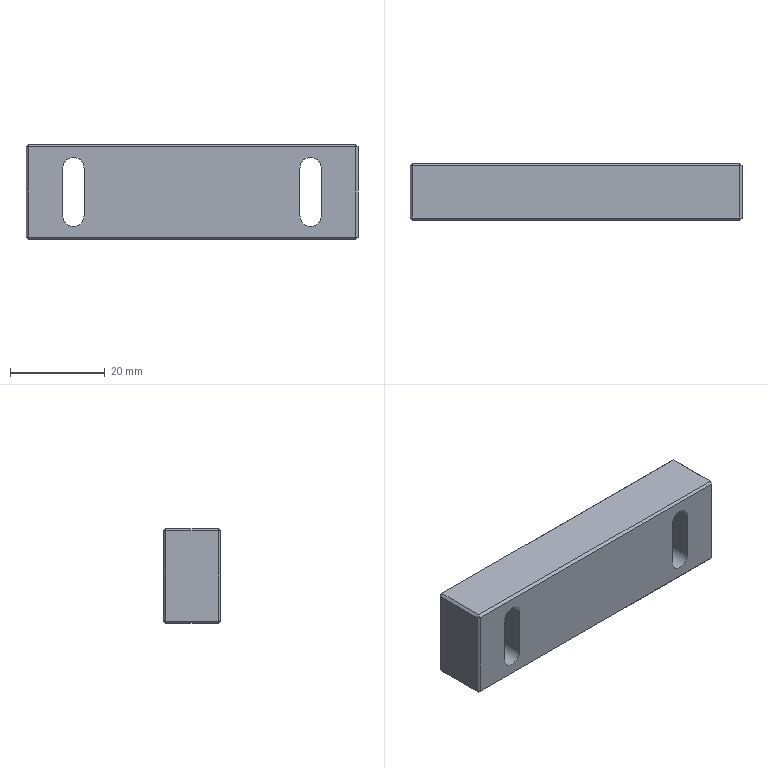Part | SolidWorks | features Chamfer 1, Cut 1, Extrusion 1 | 1 solid | 36 faces | box 70 x 12 x 20 mm | volume 15288 mm3 | plane 30 | cylinder 6 | commonest cylinder face diameters 4.5 x6
STEP:
#1=CARTESIAN_POINT('',(25.,0.,7.25));
#2=VERTEX_POINT('',#1);
#3=CARTESIAN_POINT('',(27.25,0.,5.));
#4=VERTEX_POINT('',#3);
#5=CARTESIAN_POINT('',(25.,0.,5.));
#6=DIRECTION('',(0.,1.,0.));
#7=DIRECTION('',(0.,0.,1.));
#8=AXIS2_PLACEMENT_3D('',#5,#6,#7);
#9=CIRCLE('',#8,2.25);
#10=EDGE_CURVE('',#2,#4,#9,.T.);
#11=ORIENTED_EDGE('',*,*,#10,.F.);
#12=CARTESIAN_POINT('',(25.,12.,7.25));
#13=VERTEX_POINT('',#12);
#14=CARTESIAN_POINT('',(25.,0.,7.25));
#15=DIRECTION('',(0.,1.,0.));
#16=VECTOR('',#15,1000.);
#17=LINE('',#14,#16);
#18=EDGE_CURVE('',#2,#13,#17,.T.);
#19=ORIENTED_EDGE('',*,*,#18,.T.);
#20=CARTESIAN_POINT('',(27.25,12.,5.));
#21=VERTEX_POINT('',#20);
#22=CARTESIAN_POINT('',(25.,12.,5.));
#23=DIRECTION('',(0.,1.,0.));
#24=DIRECTION('',(0.,0.,1.));
#25=AXIS2_PLACEMENT_3D('',#22,#23,#24);
#26=CIRCLE('',#25,2.25);
#27=EDGE_CURVE('',#13,#21,#26,.T.);
#28=ORIENTED_EDGE('',*,*,#27,.T.);
#29=CARTESIAN_POINT('',(27.25,0.,5.));
#30=DIRECTION('',(0.,1.,0.));
#31=VECTOR('',#30,1000.);
#32=LINE('',#29,#31);
#33=EDGE_CURVE('',#4,#21,#32,.T.);
#34=ORIENTED_EDGE('',*,*,#33,.F.);
#35=EDGE_LOOP('',(#11,#19,#28,#34));
#36=FACE_OUTER_BOUND('',#35,.T.);
#37=CARTESIAN_POINT('',(25.,0.,5.));
#38=DIRECTION('',(0.,1.,0.));
#39=DIRECTION('',(0.,0.,1.));
#40=AXIS2_PLACEMENT_3D('',#37,#38,#39);
#41=CYLINDRICAL_SURFACE('',#40,2.25);
#42=ADVANCED_FACE('',(#36),#41,.F.);
#43=CARTESIAN_POINT('',(-25.,0.,7.25));
#44=VERTEX_POINT('',#43);
#45=CARTESIAN_POINT('',(-22.75,0.,5.));
#46=VERTEX_POINT('',#45);
#47=CARTESIAN_POINT('',(-25.,0.,5.));
#48=DIRECTION('',(0.,1.,0.));
#49=DIRECTION('',(0.,0.,-1.));
#50=AXIS2_PLACEMENT_3D('',#47,#48,#49);
#51=CIRCLE('',#50,2.25);
#52=EDGE_CURVE('',#44,#46,#51,.T.);
#53=ORIENTED_EDGE('',*,*,#52,.F.);
#54=CARTESIAN_POINT('',(-25.,12.,7.25));
#55=VERTEX_POINT('',#54);
#56=CARTESIAN_POINT('',(-25.,0.,7.25));
#57=DIRECTION('',(0.,1.,0.));
#58=VECTOR('',#57,1000.);
#59=LINE('',#56,#58);
#60=EDGE_CURVE('',#44,#55,#59,.T.);
#61=ORIENTED_EDGE('',*,*,#60,.T.);
#62=CARTESIAN_POINT('',(-22.75,12.,5.));
#63=VERTEX_POINT('',#62);
#64=CARTESIAN_POINT('',(-25.,12.,5.));
#65=DIRECTION('',(0.,1.,0.));
#66=DIRECTION('',(0.,0.,-1.));
#67=AXIS2_PLACEMENT_3D('',#64,#65,#66);
#68=CIRCLE('',#67,2.25);
#69=EDGE_CURVE('',#55,#63,#68,.T.);
#70=ORIENTED_EDGE('',*,*,#69,.T.);
#71=CARTESIAN_POINT('',(-22.75,0.,5.));
#72=DIRECTION('',(0.,1.,0.));
#73=VECTOR('',#72,1000.);
#74=LINE('',#71,#73);
#75=EDGE_CURVE('',#46,#63,#74,.T.);
#76=ORIENTED_EDGE('',*,*,#75,.F.);
#77=EDGE_LOOP('',(#53,#61,#70,#76));
#78=FACE_OUTER_BOUND('',#77,.T.);
#79=CARTESIAN_POINT('',(-25.,0.,5.));
#80=DIRECTION('',(0.,1.,0.));
#81=DIRECTION('',(0.,0.,1.));
#82=AXIS2_PLACEMENT_3D('',#79,#80,#81);
#83=CYLINDRICAL_SURFACE('',#82,2.25);
#84=ADVANCED_FACE('',(#78),#83,.F.);
#85=CARTESIAN_POINT('',(-35.,11.5,9.5));
#86=VERTEX_POINT('',#85);
#87=CARTESIAN_POINT('',(-35.,11.5,-9.5));
#88=VERTEX_POINT('',#87);
#89=CARTESIAN_POINT('',(-35.,11.5,-10.));
#90=DIRECTION('',(0.,0.,-1.));
#91=VECTOR('',#90,1000.);
#92=LINE('',#89,#91);
#93=EDGE_CURVE('',#86,#88,#92,.T.);
#94=ORIENTED_EDGE('',*,*,#93,.T.);
#95=CARTESIAN_POINT('',(-35.,0.5,-9.5));
#96=VERTEX_POINT('',#95);
#97=CARTESIAN_POINT('',(-35.,12.,-9.5));
#98=DIRECTION('',(0.,-1.,0.));
#99=VECTOR('',#98,1000.);
#100=LINE('',#97,#99);
#101=EDGE_CURVE('',#88,#96,#100,.T.);
#102=ORIENTED_EDGE('',*,*,#101,.T.);
#103=CARTESIAN_POINT('',(-35.,0.5,9.5));
#104=VERTEX_POINT('',#103);
#105=CARTESIAN_POINT('',(-35.,0.5,-10.));
#106=DIRECTION('',(0.,0.,1.));
#107=VECTOR('',#106,1000.);
#108=LINE('',#105,#107);
#109=EDGE_CURVE('',#96,#104,#108,.T.);
#110=ORIENTED_EDGE('',*,*,#109,.T.);
#111=CARTESIAN_POINT('',(-35.,12.,9.5));
#112=DIRECTION('',(0.,1.,0.));
#113=VECTOR('',#112,1000.);
#114=LINE('',#111,#113);
#115=EDGE_CURVE('',#104,#86,#114,.T.);
#116=ORIENTED_EDGE('',*,*,#115,.T.);
#117=EDGE_LOOP('',(#94,#102,#110,#116));
#118=FACE_OUTER_BOUND('',#117,.T.);
#119=CARTESIAN_POINT('',(-35.,12.,-10.));
#120=DIRECTION('',(1.,0.,0.));
#121=DIRECTION('',(0.,0.,-1.));
#122=AXIS2_PLACEMENT_3D('',#119,#120,#121);
#123=PLANE('',#122);
#124=ADVANCED_FACE('',(#118),#123,.F.);
#125=CARTESIAN_POINT('',(-34.5,0.5,10.));
#126=VERTEX_POINT('',#125);
#127=CARTESIAN_POINT('',(34.5,0.5,10.));
#128=VERTEX_POINT('',#127);
#129=CARTESIAN_POINT('',(-35.,0.5,10.));
#130=DIRECTION('',(1.,0.,0.));
#131=VECTOR('',#130,1000.);
#132=LINE('',#129,#131);
#133=EDGE_CURVE('',#126,#128,#132,.T.);
#134=ORIENTED_EDGE('',*,*,#133,.T.);
#135=CARTESIAN_POINT('',(34.5,11.5,10.));
#136=VERTEX_POINT('',#135);
#137=CARTESIAN_POINT('',(34.5,12.,10.));
#138=DIRECTION('',(0.,1.,0.));
#139=VECTOR('',#138,1000.);
#140=LINE('',#137,#139);
#141=EDGE_CURVE('',#128,#136,#140,.T.);
#142=ORIENTED_EDGE('',*,*,#141,.T.);
#143=CARTESIAN_POINT('',(-34.5,11.5,10.));
#144=VERTEX_POINT('',#143);
#145=CARTESIAN_POINT('',(-35.,11.5,10.));
#146=DIRECTION('',(-1.,0.,0.));
#147=VECTOR('',#146,1000.);
#148=LINE('',#145,#147);
#149=EDGE_CURVE('',#136,#144,#148,.T.);
#150=ORIENTED_EDGE('',*,*,#149,.T.);
#151=CARTESIAN_POINT('',(-34.5,12.,10.));
#152=DIRECTION('',(0.,-1.,0.));
#153=VECTOR('',#152,1000.);
#154=LINE('',#151,#153);
#155=EDGE_CURVE('',#144,#126,#154,.T.);
#156=ORIENTED_EDGE('',*,*,#155,.T.);
#157=EDGE_LOOP('',(#134,#142,#150,#156));
#158=FACE_OUTER_BOUND('',#157,.T.);
#159=CARTESIAN_POINT('',(-35.,12.,10.));
#160=DIRECTION('',(0.,0.,-1.));
#161=DIRECTION('',(-1.,0.,0.));
#162=AXIS2_PLACEMENT_3D('',#159,#160,#161);
#163=PLANE('',#162);
#164=ADVANCED_FACE('',(#158),#163,.F.);
#165=CARTESIAN_POINT('',(35.,11.5,-9.5));
#166=VERTEX_POINT('',#165);
#167=CARTESIAN_POINT('',(35.,11.5,9.5));
#168=VERTEX_POINT('',#167);
#169=CARTESIAN_POINT('',(35.,11.5,10.));
#170=DIRECTION('',(0.,0.,1.));
#171=VECTOR('',#170,1000.);
#172=LINE('',#169,#171);
#173=EDGE_CURVE('',#166,#168,#172,.T.);
#174=ORIENTED_EDGE('',*,*,#173,.T.);
#175=CARTESIAN_POINT('',(35.,0.5,9.5));
#176=VERTEX_POINT('',#175);
#177=CARTESIAN_POINT('',(35.,12.,9.5));
#178=DIRECTION('',(0.,-1.,0.));
#179=VECTOR('',#178,1000.);
#180=LINE('',#177,#179);
#181=EDGE_CURVE('',#168,#176,#180,.T.);
#182=ORIENTED_EDGE('',*,*,#181,.T.);
#183=CARTESIAN_POINT('',(35.,0.5,-9.5));
#184=VERTEX_POINT('',#183);
#185=CARTESIAN_POINT('',(35.,0.5,-10.));
#186=DIRECTION('',(0.,0.,-1.));
#187=VECTOR('',#186,1000.);
#188=LINE('',#185,#187);
#189=EDGE_CURVE('',#176,#184,#188,.T.);
#190=ORIENTED_EDGE('',*,*,#189,.T.);
#191=CARTESIAN_POINT('',(35.,12.,-9.5));
#192=DIRECTION('',(0.,1.,0.));
#193=VECTOR('',#192,1000.);
#194=LINE('',#191,#193);
#195=EDGE_CURVE('',#184,#166,#194,.T.);
#196=ORIENTED_EDGE('',*,*,#195,.T.);
#197=EDGE_LOOP('',(#174,#182,#190,#196));
#198=FACE_OUTER_BOUND('',#197,.T.);
#199=CARTESIAN_POINT('',(35.,12.,-10.));
#200=DIRECTION('',(-1.,0.,0.));
#201=DIRECTION('',(0.,0.,1.));
#202=AXIS2_PLACEMENT_3D('',#199,#200,#201);
#203=PLANE('',#202);
#204=ADVANCED_FACE('',(#198),#203,.F.);
#205=CARTESIAN_POINT('',(-34.5,11.5,-10.));
#206=VERTEX_POINT('',#205);
#207=CARTESIAN_POINT('',(34.5,11.5,-10.));
#208=VERTEX_POINT('',#207);
#209=CARTESIAN_POINT('',(35.,11.5,-10.));
#210=DIRECTION('',(1.,0.,0.));
#211=VECTOR('',#210,1000.);
#212=LINE('',#209,#211);
#213=EDGE_CURVE('',#206,#208,#212,.T.);
#214=ORIENTED_EDGE('',*,*,#213,.T.);
#215=CARTESIAN_POINT('',(34.5,0.5,-10.));
#216=VERTEX_POINT('',#215);
#217=CARTESIAN_POINT('',(34.5,12.,-10.));
#218=DIRECTION('',(0.,-1.,0.));
#219=VECTOR('',#218,1000.);
#220=LINE('',#217,#219);
#221=EDGE_CURVE('',#208,#216,#220,.T.);
#222=ORIENTED_EDGE('',*,*,#221,.T.);
#223=CARTESIAN_POINT('',(-34.5,0.5,-10.));
#224=VERTEX_POINT('',#223);
#225=CARTESIAN_POINT('',(-35.,0.5,-10.));
#226=DIRECTION('',(-1.,0.,0.));
#227=VECTOR('',#226,1000.);
#228=LINE('',#225,#227);
#229=EDGE_CURVE('',#216,#224,#228,.T.);
#230=ORIENTED_EDGE('',*,*,#229,.T.);
#231=CARTESIAN_POINT('',(-34.5,12.,-10.));
#232=DIRECTION('',(0.,1.,0.));
#233=VECTOR('',#232,1000.);
#234=LINE('',#231,#233);
#235=EDGE_CURVE('',#224,#206,#234,.T.);
#236=ORIENTED_EDGE('',*,*,#235,.T.);
#237=EDGE_LOOP('',(#214,#222,#230,#236));
#238=FACE_OUTER_BOUND('',#237,.T.);
#239=CARTESIAN_POINT('',(-35.,12.,-10.));
#240=DIRECTION('',(0.,0.,1.));
#241=DIRECTION('',(1.,0.,0.));
#242=AXIS2_PLACEMENT_3D('',#239,#240,#241);
#243=PLANE('',#242);
#244=ADVANCED_FACE('',(#238),#243,.F.);
#245=CARTESIAN_POINT('',(-34.5,12.,-9.5));
#246=VERTEX_POINT('',#245);
#247=CARTESIAN_POINT('',(-34.5,12.,9.5));
#248=VERTEX_POINT('',#247);
#249=CARTESIAN_POINT('',(-34.5,12.,10.));
#250=DIRECTION('',(0.,0.,1.));
#251=VECTOR('',#250,1000.);
#252=LINE('',#249,#251);
#253=EDGE_CURVE('',#246,#248,#252,.T.);
#254=ORIENTED_EDGE('',*,*,#253,.T.);
#255=CARTESIAN_POINT('',(34.5,12.,9.5));
#256=VERTEX_POINT('',#255);
#257=CARTESIAN_POINT('',(35.,12.,9.5));
#258=DIRECTION('',(1.,0.,0.));
#259=VECTOR('',#258,1000.);
#260=LINE('',#257,#259);
#261=EDGE_CURVE('',#248,#256,#260,.T.);
#262=ORIENTED_EDGE('',*,*,#261,.T.);
#263=CARTESIAN_POINT('',(34.5,12.,-9.5));
#264=VERTEX_POINT('',#263);
#265=CARTESIAN_POINT('',(34.5,12.,-10.));
#266=DIRECTION('',(0.,0.,-1.));
#267=VECTOR('',#266,1000.);
#268=LINE('',#265,#267);
#269=EDGE_CURVE('',#256,#264,#268,.T.);
#270=ORIENTED_EDGE('',*,*,#269,.T.);
#271=CARTESIAN_POINT('',(-35.,12.,-9.5));
#272=DIRECTION('',(-1.,0.,0.));
#273=VECTOR('',#272,1000.);
#274=LINE('',#271,#273);
#275=EDGE_CURVE('',#264,#246,#274,.T.);
#276=ORIENTED_EDGE('',*,*,#275,.T.);
#277=EDGE_LOOP('',(#254,#262,#270,#276));
#278=FACE_OUTER_BOUND('',#277,.T.);
#279=CARTESIAN_POINT('',(22.75,12.,5.));
#280=VERTEX_POINT('',#279);
#281=CARTESIAN_POINT('',(25.,12.,5.));
#282=DIRECTION('',(0.,1.,0.));
#283=DIRECTION('',(0.,0.,1.));
#284=AXIS2_PLACEMENT_3D('',#281,#282,#283);
#285=CIRCLE('',#284,2.25);
#286=EDGE_CURVE('',#280,#13,#285,.T.);
#287=ORIENTED_EDGE('',*,*,#286,.F.);
#288=CARTESIAN_POINT('',(22.75,12.,-5.));
#289=VERTEX_POINT('',#288);
#290=CARTESIAN_POINT('',(22.75,12.,-5.));
#291=DIRECTION('',(0.,0.,1.));
#292=VECTOR('',#291,1000.);
#293=LINE('',#290,#292);
#294=EDGE_CURVE('',#289,#280,#293,.T.);
#295=ORIENTED_EDGE('',*,*,#294,.F.);
#296=CARTESIAN_POINT('',(27.25,12.,-5.));
#297=VERTEX_POINT('',#296);
#298=CARTESIAN_POINT('',(25.,12.,-5.));
#299=DIRECTION('',(0.,1.,0.));
#300=DIRECTION('',(0.,0.,1.));
#301=AXIS2_PLACEMENT_3D('',#298,#299,#300);
#302=CIRCLE('',#301,2.25);
#303=EDGE_CURVE('',#297,#289,#302,.T.);
#304=ORIENTED_EDGE('',*,*,#303,.F.);
#305=CARTESIAN_POINT('',(27.25,12.,-5.));
#306=DIRECTION('',(0.,0.,-1.));
#307=VECTOR('',#306,1000.);
#308=LINE('',#305,#307);
#309=EDGE_CURVE('',#21,#297,#308,.T.);
#310=ORIENTED_EDGE('',*,*,#309,.F.);
#311=ORIENTED_EDGE('',*,*,#27,.F.);
#312=EDGE_LOOP('',(#287,#295,#304,#310,#311));
#313=FACE_BOUND('',#312,.T.);
#314=CARTESIAN_POINT('',(-22.75,12.,-5.));
#315=VERTEX_POINT('',#314);
#316=CARTESIAN_POINT('',(-27.25,12.,-5.));
#317=VERTEX_POINT('',#316);
#318=CARTESIAN_POINT('',(-25.,12.,-5.));
#319=DIRECTION('',(0.,1.,0.));
#320=DIRECTION('',(0.,0.,-1.));
#321=AXIS2_PLACEMENT_3D('',#318,#319,#320);
#322=CIRCLE('',#321,2.25);
#323=EDGE_CURVE('',#315,#317,#322,.T.);
#324=ORIENTED_EDGE('',*,*,#323,.F.);
#325=CARTESIAN_POINT('',(-22.75,12.,-5.));
#326=DIRECTION('',(0.,0.,-1.));
#327=VECTOR('',#326,1000.);
#328=LINE('',#325,#327);
#329=EDGE_CURVE('',#63,#315,#328,.T.);
#330=ORIENTED_EDGE('',*,*,#329,.F.);
#331=ORIENTED_EDGE('',*,*,#69,.F.);
#332=CARTESIAN_POINT('',(-27.25,12.,5.));
#333=VERTEX_POINT('',#332);
#334=CARTESIAN_POINT('',(-25.,12.,5.));
#335=DIRECTION('',(0.,1.,0.));
#336=DIRECTION('',(0.,0.,-1.));
#337=AXIS2_PLACEMENT_3D('',#334,#335,#336);
#338=CIRCLE('',#337,2.25);
#339=EDGE_CURVE('',#333,#55,#338,.T.);
#340=ORIENTED_EDGE('',*,*,#339,.F.);
#341=CARTESIAN_POINT('',(-27.25,12.,-5.));
#342=DIRECTION('',(0.,0.,1.));
#343=VECTOR('',#342,1000.);
#344=LINE('',#341,#343);
#345=EDGE_CURVE('',#317,#333,#344,.T.);
#346=ORIENTED_EDGE('',*,*,#345,.F.);
#347=EDGE_LOOP('',(#324,#330,#331,#340,#346));
#348=FACE_BOUND('',#347,.T.);
#349=CARTESIAN_POINT('',(-35.,12.,10.));
#350=DIRECTION('',(0.,1.,0.));
#351=DIRECTION('',(0.,0.,1.));
#352=AXIS2_PLACEMENT_3D('',#349,#350,#351);
#353=PLANE('',#352);
#354=ADVANCED_FACE('',(#278,#313,#348),#353,.T.);
#355=CARTESIAN_POINT('',(34.5,0.,-9.5));
#356=VERTEX_POINT('',#355);
#357=CARTESIAN_POINT('',(34.5,0.,9.5));
#358=VERTEX_POINT('',#357);
#359=CARTESIAN_POINT('',(34.5,0.,10.));
#360=DIRECTION('',(0.,0.,1.));
#361=VECTOR('',#360,1000.);
#362=LINE('',#359,#361);
#363=EDGE_CURVE('',#356,#358,#362,.T.);
#364=ORIENTED_EDGE('',*,*,#363,.T.);
#365=CARTESIAN_POINT('',(-34.5,0.,9.5));
#366=VERTEX_POINT('',#365);
#367=CARTESIAN_POINT('',(-35.,0.,9.5));
#368=DIRECTION('',(-1.,0.,0.));
#369=VECTOR('',#368,1000.);
#370=LINE('',#367,#369);
#371=EDGE_CURVE('',#358,#366,#370,.T.);
#372=ORIENTED_EDGE('',*,*,#371,.T.);
#373=CARTESIAN_POINT('',(-34.5,0.,-9.5));
#374=VERTEX_POINT('',#373);
#375=CARTESIAN_POINT('',(-34.5,0.,10.));
#376=DIRECTION('',(0.,0.,-1.));
#377=VECTOR('',#376,1000.);
#378=LINE('',#375,#377);
#379=EDGE_CURVE('',#366,#374,#378,.T.);
#380=ORIENTED_EDGE('',*,*,#379,.T.);
#381=CARTESIAN_POINT('',(-35.,0.,-9.5));
#382=DIRECTION('',(1.,0.,0.));
#383=VECTOR('',#382,1000.);
#384=LINE('',#381,#383);
#385=EDGE_CURVE('',#374,#356,#384,.T.);
#386=ORIENTED_EDGE('',*,*,#385,.T.);
#387=EDGE_LOOP('',(#364,#372,#380,#386));
#388=FACE_OUTER_BOUND('',#387,.T.);
#389=CARTESIAN_POINT('',(22.75,0.,-5.));
#390=VERTEX_POINT('',#389);
#391=CARTESIAN_POINT('',(22.75,0.,5.));
#392=VERTEX_POINT('',#391);
#393=CARTESIAN_POINT('',(22.75,0.,-5.));
#394=DIRECTION('',(0.,0.,1.));
#395=VECTOR('',#394,1000.);
#396=LINE('',#393,#395);
#397=EDGE_CURVE('',#390,#392,#396,.T.);
#398=ORIENTED_EDGE('',*,*,#397,.T.);
#399=CARTESIAN_POINT('',(25.,0.,5.));
#400=DIRECTION('',(0.,1.,0.));
#401=DIRECTION('',(0.,0.,1.));
#402=AXIS2_PLACEMENT_3D('',#399,#400,#401);
#403=CIRCLE('',#402,2.25);
#404=EDGE_CURVE('',#392,#2,#403,.T.);
#405=ORIENTED_EDGE('',*,*,#404,.T.);
#406=ORIENTED_EDGE('',*,*,#10,.T.);
#407=CARTESIAN_POINT('',(27.25,0.,-5.));
#408=VERTEX_POINT('',#407);
#409=CARTESIAN_POINT('',(27.25,0.,-5.));
#410=DIRECTION('',(0.,0.,-1.));
#411=VECTOR('',#410,1000.);
#412=LINE('',#409,#411);
#413=EDGE_CURVE('',#4,#408,#412,.T.);
#414=ORIENTED_EDGE('',*,*,#413,.T.);
#415=CARTESIAN_POINT('',(25.,0.,-5.));
#416=DIRECTION('',(0.,1.,0.));
#417=DIRECTION('',(0.,0.,1.));
#418=AXIS2_PLACEMENT_3D('',#415,#416,#417);
#419=CIRCLE('',#418,2.25);
#420=EDGE_CURVE('',#408,#390,#419,.T.);
#421=ORIENTED_EDGE('',*,*,#420,.T.);
#422=EDGE_LOOP('',(#398,#405,#406,#414,#421));
#423=FACE_BOUND('',#422,.T.);
#424=CARTESIAN_POINT('',(-22.75,0.,-5.));
#425=VERTEX_POINT('',#424);
#426=CARTESIAN_POINT('',(-22.75,0.,-5.));
#427=DIRECTION('',(0.,0.,-1.));
#428=VECTOR('',#427,1000.);
#429=LINE('',#426,#428);
#430=EDGE_CURVE('',#46,#425,#429,.T.);
#431=ORIENTED_EDGE('',*,*,#430,.T.);
#432=CARTESIAN_POINT('',(-27.25,0.,-5.));
#433=VERTEX_POINT('',#432);
#434=CARTESIAN_POINT('',(-25.,0.,-5.));
#435=DIRECTION('',(0.,1.,0.));
#436=DIRECTION('',(0.,0.,-1.));
#437=AXIS2_PLACEMENT_3D('',#434,#435,#436);
#438=CIRCLE('',#437,2.25);
#439=EDGE_CURVE('',#425,#433,#438,.T.);
#440=ORIENTED_EDGE('',*,*,#439,.T.);
#441=CARTESIAN_POINT('',(-27.25,0.,5.));
#442=VERTEX_POINT('',#441);
#443=CARTESIAN_POINT('',(-27.25,0.,-5.));
#444=DIRECTION('',(0.,0.,1.));
#445=VECTOR('',#444,1000.);
#446=LINE('',#443,#445);
#447=EDGE_CURVE('',#433,#442,#446,.T.);
#448=ORIENTED_EDGE('',*,*,#447,.T.);
#449=CARTESIAN_POINT('',(-25.,0.,5.));
#450=DIRECTION('',(0.,1.,0.));
#451=DIRECTION('',(0.,0.,-1.));
#452=AXIS2_PLACEMENT_3D('',#449,#450,#451);
#453=CIRCLE('',#452,2.25);
#454=EDGE_CURVE('',#442,#44,#453,.T.);
#455=ORIENTED_EDGE('',*,*,#454,.T.);
#456=ORIENTED_EDGE('',*,*,#52,.T.);
#457=EDGE_LOOP('',(#431,#440,#448,#455,#456));
#458=FACE_BOUND('',#457,.T.);
#459=CARTESIAN_POINT('',(-35.,0.,10.));
#460=DIRECTION('',(0.,1.,0.));
#461=DIRECTION('',(0.,0.,1.));
#462=AXIS2_PLACEMENT_3D('',#459,#460,#461);
#463=PLANE('',#462);
#464=ADVANCED_FACE('',(#388,#423,#458),#463,.F.);
#465=ORIENTED_EDGE('',*,*,#323,.T.);
#466=CARTESIAN_POINT('',(-27.25,0.,-5.));
#467=DIRECTION('',(0.,1.,0.));
#468=VECTOR('',#467,1000.);
#469=LINE('',#466,#468);
#470=EDGE_CURVE('',#433,#317,#469,.T.);
#471=ORIENTED_EDGE('',*,*,#470,.F.);
#472=ORIENTED_EDGE('',*,*,#439,.F.);
#473=CARTESIAN_POINT('',(-22.75,0.,-5.));
#474=DIRECTION('',(0.,1.,0.));
#475=VECTOR('',#474,1000.);
#476=LINE('',#473,#475);
#477=EDGE_CURVE('',#425,#315,#476,.T.);
#478=ORIENTED_EDGE('',*,*,#477,.T.);
#479=EDGE_LOOP('',(#465,#471,#472,#478));
#480=FACE_OUTER_BOUND('',#479,.T.);
#481=CARTESIAN_POINT('',(-25.,0.,-5.));
#482=DIRECTION('',(0.,1.,0.));
#483=DIRECTION('',(0.,0.,1.));
#484=AXIS2_PLACEMENT_3D('',#481,#482,#483);
#485=CYLINDRICAL_SURFACE('',#484,2.25);
#486=ADVANCED_FACE('',(#480),#485,.F.);
#487=ORIENTED_EDGE('',*,*,#329,.T.);
#488=ORIENTED_EDGE('',*,*,#477,.F.);
#489=ORIENTED_EDGE('',*,*,#430,.F.);
#490=ORIENTED_EDGE('',*,*,#75,.T.);
#491=EDGE_LOOP('',(#487,#488,#489,#490));
#492=FACE_OUTER_BOUND('',#491,.T.);
#493=CARTESIAN_POINT('',(-22.75,0.,-5.));
#494=DIRECTION('',(1.,0.,0.));
#495=DIRECTION('',(0.,0.,-1.));
#496=AXIS2_PLACEMENT_3D('',#493,#494,#495);
#497=PLANE('',#496);
#498=ADVANCED_FACE('',(#492),#497,.F.);
#499=ORIENTED_EDGE('',*,*,#60,.F.);
#500=ORIENTED_EDGE('',*,*,#454,.F.);
#501=CARTESIAN_POINT('',(-27.25,0.,5.));
#502=DIRECTION('',(0.,1.,0.));
#503=VECTOR('',#502,1000.);
#504=LINE('',#501,#503);
#505=EDGE_CURVE('',#442,#333,#504,.T.);
#506=ORIENTED_EDGE('',*,*,#505,.T.);
#507=ORIENTED_EDGE('',*,*,#339,.T.);
#508=EDGE_LOOP('',(#499,#500,#506,#507));
#509=FACE_OUTER_BOUND('',#508,.T.);
#510=CARTESIAN_POINT('',(-25.,0.,5.));
#511=DIRECTION('',(0.,1.,0.));
#512=DIRECTION('',(0.,0.,1.));
#513=AXIS2_PLACEMENT_3D('',#510,#511,#512);
#514=CYLINDRICAL_SURFACE('',#513,2.25);
#515=ADVANCED_FACE('',(#509),#514,.F.);
#516=ORIENTED_EDGE('',*,*,#345,.T.);
#517=ORIENTED_EDGE('',*,*,#505,.F.);
#518=ORIENTED_EDGE('',*,*,#447,.F.);
#519=ORIENTED_EDGE('',*,*,#470,.T.);
#520=EDGE_LOOP('',(#516,#517,#518,#519));
#521=FACE_OUTER_BOUND('',#520,.T.);
#522=CARTESIAN_POINT('',(-27.25,0.,-5.));
#523=DIRECTION('',(-1.,0.,0.));
#524=DIRECTION('',(0.,0.,1.));
#525=AXIS2_PLACEMENT_3D('',#522,#523,#524);
#526=PLANE('',#525);
#527=ADVANCED_FACE('',(#521),#526,.F.);
#528=ORIENTED_EDGE('',*,*,#18,.F.);
#529=ORIENTED_EDGE('',*,*,#404,.F.);
#530=CARTESIAN_POINT('',(22.75,0.,5.));
#531=DIRECTION('',(0.,1.,0.));
#532=VECTOR('',#531,1000.);
#533=LINE('',#530,#532);
#534=EDGE_CURVE('',#392,#280,#533,.T.);
#535=ORIENTED_EDGE('',*,*,#534,.T.);
#536=ORIENTED_EDGE('',*,*,#286,.T.);
#537=EDGE_LOOP('',(#528,#529,#535,#536));
#538=FACE_OUTER_BOUND('',#537,.T.);
#539=CARTESIAN_POINT('',(25.,0.,5.));
#540=DIRECTION('',(0.,1.,0.));
#541=DIRECTION('',(0.,0.,1.));
#542=AXIS2_PLACEMENT_3D('',#539,#540,#541);
#543=CYLINDRICAL_SURFACE('',#542,2.25);
#544=ADVANCED_FACE('',(#538),#543,.F.);
#545=ORIENTED_EDGE('',*,*,#294,.T.);
#546=ORIENTED_EDGE('',*,*,#534,.F.);
#547=ORIENTED_EDGE('',*,*,#397,.F.);
#548=CARTESIAN_POINT('',(22.75,0.,-5.));
#549=DIRECTION('',(0.,1.,0.));
#550=VECTOR('',#549,1000.);
#551=LINE('',#548,#550);
#552=EDGE_CURVE('',#390,#289,#551,.T.);
#553=ORIENTED_EDGE('',*,*,#552,.T.);
#554=EDGE_LOOP('',(#545,#546,#547,#553));
#555=FACE_OUTER_BOUND('',#554,.T.);
#556=CARTESIAN_POINT('',(22.75,0.,-5.));
#557=DIRECTION('',(-1.,0.,0.));
#558=DIRECTION('',(0.,0.,1.));
#559=AXIS2_PLACEMENT_3D('',#556,#557,#558);
#560=PLANE('',#559);
#561=ADVANCED_FACE('',(#555),#560,.F.);
#562=ORIENTED_EDGE('',*,*,#303,.T.);
#563=ORIENTED_EDGE('',*,*,#552,.F.);
#564=ORIENTED_EDGE('',*,*,#420,.F.);
#565=CARTESIAN_POINT('',(27.25,0.,-5.));
#566=DIRECTION('',(0.,1.,0.));
#567=VECTOR('',#566,1000.);
#568=LINE('',#565,#567);
#569=EDGE_CURVE('',#408,#297,#568,.T.);
#570=ORIENTED_EDGE('',*,*,#569,.T.);
#571=EDGE_LOOP('',(#562,#563,#564,#570));
#572=FACE_OUTER_BOUND('',#571,.T.);
#573=CARTESIAN_POINT('',(25.,0.,-5.));
#574=DIRECTION('',(0.,1.,0.));
#575=DIRECTION('',(0.,0.,1.));
#576=AXIS2_PLACEMENT_3D('',#573,#574,#575);
#577=CYLINDRICAL_SURFACE('',#576,2.25);
#578=ADVANCED_FACE('',(#572),#577,.F.);
#579=ORIENTED_EDGE('',*,*,#309,.T.);
#580=ORIENTED_EDGE('',*,*,#569,.F.);
#581=ORIENTED_EDGE('',*,*,#413,.F.);
#582=ORIENTED_EDGE('',*,*,#33,.T.);
#583=EDGE_LOOP('',(#579,#580,#581,#582));
#584=FACE_OUTER_BOUND('',#583,.T.);
#585=CARTESIAN_POINT('',(27.25,0.,-5.));
#586=DIRECTION('',(1.,0.,0.));
#587=DIRECTION('',(0.,0.,-1.));
#588=AXIS2_PLACEMENT_3D('',#585,#586,#587);
#589=PLANE('',#588);
#590=ADVANCED_FACE('',(#584),#589,.F.);
#591=CARTESIAN_POINT('',(-34.5,0.5,-10.));
#592=DIRECTION('',(0.,-0.7071,0.7071));
#593=VECTOR('',#592,1000.);
#594=LINE('',#591,#593);
#595=EDGE_CURVE('',#224,#374,#594,.T.);
#596=ORIENTED_EDGE('',*,*,#595,.F.);
#597=ORIENTED_EDGE('',*,*,#229,.F.);
#598=CARTESIAN_POINT('',(34.5,0.25,-9.75));
#599=DIRECTION('',(0.,0.7071,-0.7071));
#600=VECTOR('',#599,1000.);
#601=LINE('',#598,#600);
#602=EDGE_CURVE('',#356,#216,#601,.T.);
#603=ORIENTED_EDGE('',*,*,#602,.F.);
#604=ORIENTED_EDGE('',*,*,#385,.F.);
#605=EDGE_LOOP('',(#596,#597,#603,#604));
#606=FACE_OUTER_BOUND('',#605,.T.);
#607=CARTESIAN_POINT('',(-35.,0.5,-10.));
#608=DIRECTION('',(0.,0.7071,0.7071));
#609=DIRECTION('',(0.,-0.7071,0.7071));
#610=AXIS2_PLACEMENT_3D('',#607,#608,#609);
#611=PLANE('',#610);
#612=ADVANCED_FACE('',(#606),#611,.F.);
#613=CARTESIAN_POINT('',(-34.5,0.5,-10.));
#614=DIRECTION('',(-0.7071,0.,0.7071));
#615=VECTOR('',#614,1000.);
#616=LINE('',#613,#615);
#617=EDGE_CURVE('',#224,#96,#616,.T.);
#618=ORIENTED_EDGE('',*,*,#617,.F.);
#619=ORIENTED_EDGE('',*,*,#595,.T.);
#620=CARTESIAN_POINT('',(-34.75,0.25,-9.5));
#621=DIRECTION('',(0.7071,-0.7071,0.));
#622=VECTOR('',#621,1000.);
#623=LINE('',#620,#622);
#624=EDGE_CURVE('',#96,#374,#623,.T.);
#625=ORIENTED_EDGE('',*,*,#624,.F.);
#626=EDGE_LOOP('',(#618,#619,#625));
#627=FACE_OUTER_BOUND('',#626,.T.);
#628=CARTESIAN_POINT('',(-34.5,0.5,-10.));
#629=DIRECTION('',(-0.5774,-0.5774,-0.5774));
#630=DIRECTION('',(-0.7071,0.,0.7071));
#631=AXIS2_PLACEMENT_3D('',#628,#629,#630);
#632=PLANE('',#631);
#633=ADVANCED_FACE('',(#627),#632,.T.);
#634=CARTESIAN_POINT('',(35.,0.5,-9.5));
#635=DIRECTION('',(0.7071,0.7071,0.));
#636=VECTOR('',#635,1000.);
#637=LINE('',#634,#636);
#638=EDGE_CURVE('',#356,#184,#637,.T.);
#639=ORIENTED_EDGE('',*,*,#638,.F.);
#640=ORIENTED_EDGE('',*,*,#602,.T.);
#641=CARTESIAN_POINT('',(35.,0.5,-9.5));
#642=DIRECTION('',(-0.7071,0.,-0.7071));
#643=VECTOR('',#642,1000.);
#644=LINE('',#641,#643);
#645=EDGE_CURVE('',#184,#216,#644,.T.);
#646=ORIENTED_EDGE('',*,*,#645,.F.);
#647=EDGE_LOOP('',(#639,#640,#646));
#648=FACE_OUTER_BOUND('',#647,.T.);
#649=CARTESIAN_POINT('',(35.,0.5,-9.5));
#650=DIRECTION('',(0.5774,-0.5774,-0.5774));
#651=DIRECTION('',(0.7071,0.7071,0.));
#652=AXIS2_PLACEMENT_3D('',#649,#650,#651);
#653=PLANE('',#652);
#654=ADVANCED_FACE('',(#648),#653,.T.);
#655=ORIENTED_EDGE('',*,*,#624,.T.);
#656=ORIENTED_EDGE('',*,*,#379,.F.);
#657=CARTESIAN_POINT('',(-34.5,0.,9.5));
#658=DIRECTION('',(0.7071,-0.7071,0.));
#659=VECTOR('',#658,1000.);
#660=LINE('',#657,#659);
#661=EDGE_CURVE('',#104,#366,#660,.T.);
#662=ORIENTED_EDGE('',*,*,#661,.F.);
#663=ORIENTED_EDGE('',*,*,#109,.F.);
#664=EDGE_LOOP('',(#655,#656,#662,#663));
#665=FACE_OUTER_BOUND('',#664,.T.);
#666=CARTESIAN_POINT('',(-35.,0.5,-10.));
#667=DIRECTION('',(0.7071,0.7071,0.));
#668=DIRECTION('',(-0.7071,0.7071,0.));
#669=AXIS2_PLACEMENT_3D('',#666,#667,#668);
#670=PLANE('',#669);
#671=ADVANCED_FACE('',(#665),#670,.F.);
#672=ORIENTED_EDGE('',*,*,#617,.T.);
#673=ORIENTED_EDGE('',*,*,#101,.F.);
#674=CARTESIAN_POINT('',(-34.75,11.5,-9.75));
#675=DIRECTION('',(-0.7071,0.,0.7071));
#676=VECTOR('',#675,1000.);
#677=LINE('',#674,#676);
#678=EDGE_CURVE('',#206,#88,#677,.T.);
#679=ORIENTED_EDGE('',*,*,#678,.F.);
#680=ORIENTED_EDGE('',*,*,#235,.F.);
#681=EDGE_LOOP('',(#672,#673,#679,#680));
#682=FACE_OUTER_BOUND('',#681,.T.);
#683=CARTESIAN_POINT('',(-35.,12.,-9.5));
#684=DIRECTION('',(0.7071,0.,0.7071));
#685=DIRECTION('',(0.7071,0.,-0.7071));
#686=AXIS2_PLACEMENT_3D('',#683,#684,#685);
#687=PLANE('',#686);
#688=ADVANCED_FACE('',(#682),#687,.F.);
#689=CARTESIAN_POINT('',(34.5,12.,-9.5));
#690=DIRECTION('',(0.,0.7071,0.7071));
#691=VECTOR('',#690,1000.);
#692=LINE('',#689,#691);
#693=EDGE_CURVE('',#208,#264,#692,.T.);
#694=ORIENTED_EDGE('',*,*,#693,.F.);
#695=ORIENTED_EDGE('',*,*,#213,.F.);
#696=CARTESIAN_POINT('',(-34.5,12.,-9.5));
#697=DIRECTION('',(0.,-0.7071,-0.7071));
#698=VECTOR('',#697,1000.);
#699=LINE('',#696,#698);
#700=EDGE_CURVE('',#246,#206,#699,.T.);
#701=ORIENTED_EDGE('',*,*,#700,.F.);
#702=ORIENTED_EDGE('',*,*,#275,.F.);
#703=EDGE_LOOP('',(#694,#695,#701,#702));
#704=FACE_OUTER_BOUND('',#703,.T.);
#705=CARTESIAN_POINT('',(-35.,12.,-9.5));
#706=DIRECTION('',(0.,0.7071,-0.7071));
#707=DIRECTION('',(0.,0.7071,0.7071));
#708=AXIS2_PLACEMENT_3D('',#705,#706,#707);
#709=PLANE('',#708);
#710=ADVANCED_FACE('',(#704),#709,.T.);
#711=ORIENTED_EDGE('',*,*,#645,.T.);
#712=ORIENTED_EDGE('',*,*,#221,.F.);
#713=CARTESIAN_POINT('',(34.75,11.5,-9.75));
#714=DIRECTION('',(-0.7071,0.,-0.7071));
#715=VECTOR('',#714,1000.);
#716=LINE('',#713,#715);
#717=EDGE_CURVE('',#166,#208,#716,.T.);
#718=ORIENTED_EDGE('',*,*,#717,.F.);
#719=ORIENTED_EDGE('',*,*,#195,.F.);
#720=EDGE_LOOP('',(#711,#712,#718,#719));
#721=FACE_OUTER_BOUND('',#720,.T.);
#722=CARTESIAN_POINT('',(34.5,12.,-10.));
#723=DIRECTION('',(-0.7071,0.,0.7071));
#724=DIRECTION('',(0.7071,0.,0.7071));
#725=AXIS2_PLACEMENT_3D('',#722,#723,#724);
#726=PLANE('',#725);
#727=ADVANCED_FACE('',(#721),#726,.F.);
#728=ORIENTED_EDGE('',*,*,#638,.T.);
#729=ORIENTED_EDGE('',*,*,#189,.F.);
#730=CARTESIAN_POINT('',(34.75,0.25,9.5));
#731=DIRECTION('',(0.7071,0.7071,0.));
#732=VECTOR('',#731,1000.);
#733=LINE('',#730,#732);
#734=EDGE_CURVE('',#358,#176,#733,.T.);
#735=ORIENTED_EDGE('',*,*,#734,.F.);
#736=ORIENTED_EDGE('',*,*,#363,.F.);
#737=EDGE_LOOP('',(#728,#729,#735,#736));
#738=FACE_OUTER_BOUND('',#737,.T.);
#739=CARTESIAN_POINT('',(35.,0.5,-10.));
#740=DIRECTION('',(-0.7071,0.7071,0.));
#741=DIRECTION('',(-0.7071,-0.7071,0.));
#742=AXIS2_PLACEMENT_3D('',#739,#740,#741);
#743=PLANE('',#742);
#744=ADVANCED_FACE('',(#738),#743,.F.);
#745=CARTESIAN_POINT('',(-34.5,0.,9.5));
#746=DIRECTION('',(0.,0.7071,0.7071));
#747=VECTOR('',#746,1000.);
#748=LINE('',#745,#747);
#749=EDGE_CURVE('',#366,#126,#748,.T.);
#750=ORIENTED_EDGE('',*,*,#749,.F.);
#751=ORIENTED_EDGE('',*,*,#371,.F.);
#752=CARTESIAN_POINT('',(34.5,0.5,10.));
#753=DIRECTION('',(0.,-0.7071,-0.7071));
#754=VECTOR('',#753,1000.);
#755=LINE('',#752,#754);
#756=EDGE_CURVE('',#128,#358,#755,.T.);
#757=ORIENTED_EDGE('',*,*,#756,.F.);
#758=ORIENTED_EDGE('',*,*,#133,.F.);
#759=EDGE_LOOP('',(#750,#751,#757,#758));
#760=FACE_OUTER_BOUND('',#759,.T.);
#761=CARTESIAN_POINT('',(-35.,0.5,10.));
#762=DIRECTION('',(0.,0.7071,-0.7071));
#763=DIRECTION('',(0.,0.7071,0.7071));
#764=AXIS2_PLACEMENT_3D('',#761,#762,#763);
#765=PLANE('',#764);
#766=ADVANCED_FACE('',(#760),#765,.F.);
#767=ORIENTED_EDGE('',*,*,#661,.T.);
#768=ORIENTED_EDGE('',*,*,#749,.T.);
#769=CARTESIAN_POINT('',(-34.75,0.5,9.75));
#770=DIRECTION('',(0.7071,0.,0.7071));
#771=VECTOR('',#770,1000.);
#772=LINE('',#769,#771);
#773=EDGE_CURVE('',#104,#126,#772,.T.);
#774=ORIENTED_EDGE('',*,*,#773,.F.);
#775=EDGE_LOOP('',(#767,#768,#774));
#776=FACE_OUTER_BOUND('',#775,.T.);
#777=CARTESIAN_POINT('',(-34.5,0.,9.5));
#778=DIRECTION('',(-0.5774,-0.5774,0.5774));
#779=DIRECTION('',(0.7071,0.,0.7071));
#780=AXIS2_PLACEMENT_3D('',#777,#778,#779);
#781=PLANE('',#780);
#782=ADVANCED_FACE('',(#776),#781,.T.);
#783=ORIENTED_EDGE('',*,*,#700,.T.);
#784=ORIENTED_EDGE('',*,*,#678,.T.);
#785=CARTESIAN_POINT('',(-34.5,12.,-9.5));
#786=DIRECTION('',(-0.7071,-0.7071,0.));
#787=VECTOR('',#786,1000.);
#788=LINE('',#785,#787);
#789=EDGE_CURVE('',#246,#88,#788,.T.);
#790=ORIENTED_EDGE('',*,*,#789,.F.);
#791=EDGE_LOOP('',(#783,#784,#790));
#792=FACE_OUTER_BOUND('',#791,.T.);
#793=CARTESIAN_POINT('',(-34.5,12.,-9.5));
#794=DIRECTION('',(-0.5774,0.5774,-0.5774));
#795=DIRECTION('',(-0.7071,0.,0.7071));
#796=AXIS2_PLACEMENT_3D('',#793,#794,#795);
#797=PLANE('',#796);
#798=ADVANCED_FACE('',(#792),#797,.T.);
#799=ORIENTED_EDGE('',*,*,#717,.T.);
#800=ORIENTED_EDGE('',*,*,#693,.T.);
#801=CARTESIAN_POINT('',(34.5,12.,-9.5));
#802=DIRECTION('',(-0.7071,0.7071,0.));
#803=VECTOR('',#802,1000.);
#804=LINE('',#801,#803);
#805=EDGE_CURVE('',#166,#264,#804,.T.);
#806=ORIENTED_EDGE('',*,*,#805,.F.);
#807=EDGE_LOOP('',(#799,#800,#806));
#808=FACE_OUTER_BOUND('',#807,.T.);
#809=CARTESIAN_POINT('',(34.5,12.,-9.5));
#810=DIRECTION('',(0.5774,0.5774,-0.5774));
#811=DIRECTION('',(-0.7071,0.7071,0.));
#812=AXIS2_PLACEMENT_3D('',#809,#810,#811);
#813=PLANE('',#812);
#814=ADVANCED_FACE('',(#808),#813,.T.);
#815=ORIENTED_EDGE('',*,*,#756,.T.);
#816=ORIENTED_EDGE('',*,*,#734,.T.);
#817=CARTESIAN_POINT('',(34.5,0.5,10.));
#818=DIRECTION('',(0.7071,0.,-0.7071));
#819=VECTOR('',#818,1000.);
#820=LINE('',#817,#819);
#821=EDGE_CURVE('',#128,#176,#820,.T.);
#822=ORIENTED_EDGE('',*,*,#821,.F.);
#823=EDGE_LOOP('',(#815,#816,#822));
#824=FACE_OUTER_BOUND('',#823,.T.);
#825=CARTESIAN_POINT('',(34.5,0.5,10.));
#826=DIRECTION('',(0.5774,-0.5774,0.5774));
#827=DIRECTION('',(0.7071,0.7071,0.));
#828=AXIS2_PLACEMENT_3D('',#825,#826,#827);
#829=PLANE('',#828);
#830=ADVANCED_FACE('',(#824),#829,.T.);
#831=ORIENTED_EDGE('',*,*,#773,.T.);
#832=ORIENTED_EDGE('',*,*,#155,.F.);
#833=CARTESIAN_POINT('',(-34.5,11.5,10.));
#834=DIRECTION('',(0.7071,0.,0.7071));
#835=VECTOR('',#834,1000.);
#836=LINE('',#833,#835);
#837=EDGE_CURVE('',#86,#144,#836,.T.);
#838=ORIENTED_EDGE('',*,*,#837,.F.);
#839=ORIENTED_EDGE('',*,*,#115,.F.);
#840=EDGE_LOOP('',(#831,#832,#838,#839));
#841=FACE_OUTER_BOUND('',#840,.T.);
#842=CARTESIAN_POINT('',(-34.5,12.,10.));
#843=DIRECTION('',(0.7071,0.,-0.7071));
#844=DIRECTION('',(-0.7071,0.,-0.7071));
#845=AXIS2_PLACEMENT_3D('',#842,#843,#844);
#846=PLANE('',#845);
#847=ADVANCED_FACE('',(#841),#846,.F.);
#848=ORIENTED_EDGE('',*,*,#789,.T.);
#849=ORIENTED_EDGE('',*,*,#93,.F.);
#850=CARTESIAN_POINT('',(-34.75,11.75,9.5));
#851=DIRECTION('',(-0.7071,-0.7071,0.));
#852=VECTOR('',#851,1000.);
#853=LINE('',#850,#852);
#854=EDGE_CURVE('',#248,#86,#853,.T.);
#855=ORIENTED_EDGE('',*,*,#854,.F.);
#856=ORIENTED_EDGE('',*,*,#253,.F.);
#857=EDGE_LOOP('',(#848,#849,#855,#856));
#858=FACE_OUTER_BOUND('',#857,.T.);
#859=CARTESIAN_POINT('',(-34.5,12.,10.));
#860=DIRECTION('',(-0.7071,0.7071,0.));
#861=DIRECTION('',(-0.7071,-0.7071,0.));
#862=AXIS2_PLACEMENT_3D('',#859,#860,#861);
#863=PLANE('',#862);
#864=ADVANCED_FACE('',(#858),#863,.T.);
#865=ORIENTED_EDGE('',*,*,#805,.T.);
#866=ORIENTED_EDGE('',*,*,#269,.F.);
#867=CARTESIAN_POINT('',(34.5,12.,9.5));
#868=DIRECTION('',(-0.7071,0.7071,0.));
#869=VECTOR('',#868,1000.);
#870=LINE('',#867,#869);
#871=EDGE_CURVE('',#168,#256,#870,.T.);
#872=ORIENTED_EDGE('',*,*,#871,.F.);
#873=ORIENTED_EDGE('',*,*,#173,.F.);
#874=EDGE_LOOP('',(#865,#866,#872,#873));
#875=FACE_OUTER_BOUND('',#874,.T.);
#876=CARTESIAN_POINT('',(34.5,12.,10.));
#877=DIRECTION('',(0.7071,0.7071,0.));
#878=DIRECTION('',(-0.7071,0.7071,0.));
#879=AXIS2_PLACEMENT_3D('',#876,#877,#878);
#880=PLANE('',#879);
#881=ADVANCED_FACE('',(#875),#880,.T.);
#882=ORIENTED_EDGE('',*,*,#821,.T.);
#883=ORIENTED_EDGE('',*,*,#181,.F.);
#884=CARTESIAN_POINT('',(34.75,11.5,9.75));
#885=DIRECTION('',(0.7071,0.,-0.7071));
#886=VECTOR('',#885,1000.);
#887=LINE('',#884,#886);
#888=EDGE_CURVE('',#136,#168,#887,.T.);
#889=ORIENTED_EDGE('',*,*,#888,.F.);
#890=ORIENTED_EDGE('',*,*,#141,.F.);
#891=EDGE_LOOP('',(#882,#883,#889,#890));
#892=FACE_OUTER_BOUND('',#891,.T.);
#893=CARTESIAN_POINT('',(35.,12.,9.5));
#894=DIRECTION('',(-0.7071,0.,-0.7071));
#895=DIRECTION('',(-0.7071,0.,0.7071));
#896=AXIS2_PLACEMENT_3D('',#893,#894,#895);
#897=PLANE('',#896);
#898=ADVANCED_FACE('',(#892),#897,.F.);
#899=ORIENTED_EDGE('',*,*,#854,.T.);
#900=ORIENTED_EDGE('',*,*,#837,.T.);
#901=CARTESIAN_POINT('',(-34.5,11.5,10.));
#902=DIRECTION('',(0.,-0.7071,0.7071));
#903=VECTOR('',#902,1000.);
#904=LINE('',#901,#903);
#905=EDGE_CURVE('',#248,#144,#904,.T.);
#906=ORIENTED_EDGE('',*,*,#905,.F.);
#907=EDGE_LOOP('',(#899,#900,#906));
#908=FACE_OUTER_BOUND('',#907,.T.);
#909=CARTESIAN_POINT('',(-34.5,11.5,10.));
#910=DIRECTION('',(-0.5774,0.5774,0.5774));
#911=DIRECTION('',(0.7071,0.,0.7071));
#912=AXIS2_PLACEMENT_3D('',#909,#910,#911);
#913=PLANE('',#912);
#914=ADVANCED_FACE('',(#908),#913,.T.);
#915=ORIENTED_EDGE('',*,*,#888,.T.);
#916=ORIENTED_EDGE('',*,*,#871,.T.);
#917=CARTESIAN_POINT('',(34.5,12.,9.5));
#918=DIRECTION('',(0.,0.7071,-0.7071));
#919=VECTOR('',#918,1000.);
#920=LINE('',#917,#919);
#921=EDGE_CURVE('',#136,#256,#920,.T.);
#922=ORIENTED_EDGE('',*,*,#921,.F.);
#923=EDGE_LOOP('',(#915,#916,#922));
#924=FACE_OUTER_BOUND('',#923,.T.);
#925=CARTESIAN_POINT('',(34.5,12.,9.5));
#926=DIRECTION('',(0.5774,0.5774,0.5774));
#927=DIRECTION('',(-0.7071,0.7071,0.));
#928=AXIS2_PLACEMENT_3D('',#925,#926,#927);
#929=PLANE('',#928);
#930=ADVANCED_FACE('',(#924),#929,.T.);
#931=ORIENTED_EDGE('',*,*,#905,.T.);
#932=ORIENTED_EDGE('',*,*,#149,.F.);
#933=ORIENTED_EDGE('',*,*,#921,.T.);
#934=ORIENTED_EDGE('',*,*,#261,.F.);
#935=EDGE_LOOP('',(#931,#932,#933,#934));
#936=FACE_OUTER_BOUND('',#935,.T.);
#937=CARTESIAN_POINT('',(-35.,12.,9.5));
#938=DIRECTION('',(0.,0.7071,0.7071));
#939=DIRECTION('',(0.,-0.7071,0.7071));
#940=AXIS2_PLACEMENT_3D('',#937,#938,#939);
#941=PLANE('',#940);
#942=ADVANCED_FACE('',(#936),#941,.T.);
#943=CLOSED_SHELL('',(#42,#84,#124,#164,#204,#244,#354,#464,#486,#498,#515,#527,#544,#561,#578,#590,#612,#633,#654,#671,#688,#710,#727,#744,#766,#782,#798,#814,#830,#847,#864,#881,#898,#914,#930,#942));
#944=MANIFOLD_SOLID_BREP('',#943);
#945=CARTESIAN_POINT('',(0.,0.,0.));
#946=DIRECTION('',(0.,0.,1.));
#947=DIRECTION('',(1.,0.,0.));
#948=AXIS2_PLACEMENT_3D('',#945,#946,#947);
#949=(LENGTH_UNIT()NAMED_UNIT(*)SI_UNIT(.MILLI.,.METRE.));
#950=UNCERTAINTY_MEASURE_WITH_UNIT(LENGTH_MEASURE(0.00001),#949,'','');
#951=(NAMED_UNIT(*)PLANE_ANGLE_UNIT()SI_UNIT($,.RADIAN.));
#952=(NAMED_UNIT(*)SI_UNIT($,.STERADIAN.)SOLID_ANGLE_UNIT());
#953=(GEOMETRIC_REPRESENTATION_CONTEXT(3)GLOBAL_UNCERTAINTY_ASSIGNED_CONTEXT((#950))GLOBAL_UNIT_ASSIGNED_CONTEXT((#949,#951,#952))REPRESENTATION_CONTEXT('',''));
#954=ADVANCED_BREP_SHAPE_REPRESENTATION('',(#944,#948),#953);